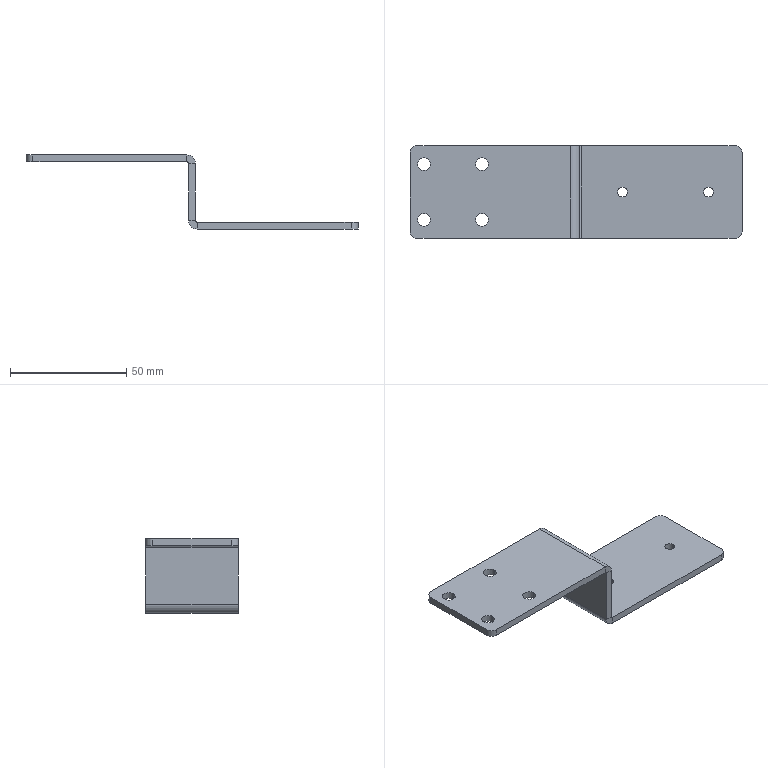Part | SolidWorks | features HoleWzd 2, Fillet 1, FlatPattern 1, SMBaseFlange 1, SheetMetal 1 | 1 solid | 38 faces | box 143 x 40 x 32 mm | volume 20017 mm3 | cylinder 20 | plane 18 | commonest cylinder face diameters 5.5 x8 4.2 x4 6 x4 1.5 x2 7.5 x2
STEP:
#1=CARTESIAN_POINT('',(8.75,8.,0.));
#2=VERTEX_POINT('',#1);
#3=CARTESIAN_POINT('',(3.25,8.,0.));
#4=VERTEX_POINT('',#3);
#5=CARTESIAN_POINT('',(6.,8.,0.));
#6=DIRECTION('',(0.,0.,-1.));
#7=DIRECTION('',(-1.,0.,0.));
#8=AXIS2_PLACEMENT_3D('',#5,#6,#7);
#9=CIRCLE('',#8,2.75);
#10=EDGE_CURVE('',#2,#4,#9,.T.);
#11=ORIENTED_EDGE('',*,*,#10,.T.);
#12=CARTESIAN_POINT('',(3.25,8.,3.));
#13=VERTEX_POINT('',#12);
#14=CARTESIAN_POINT('',(3.25,8.,3.));
#15=DIRECTION('',(0.,0.,1.));
#16=VECTOR('',#15,1000.);
#17=LINE('',#14,#16);
#18=EDGE_CURVE('',#4,#13,#17,.T.);
#19=ORIENTED_EDGE('',*,*,#18,.T.);
#20=CARTESIAN_POINT('',(8.75,8.,3.));
#21=VERTEX_POINT('',#20);
#22=CARTESIAN_POINT('',(6.,8.,3.));
#23=DIRECTION('',(0.,0.,1.));
#24=DIRECTION('',(1.,0.,0.));
#25=AXIS2_PLACEMENT_3D('',#22,#23,#24);
#26=CIRCLE('',#25,2.75);
#27=EDGE_CURVE('',#13,#21,#26,.T.);
#28=ORIENTED_EDGE('',*,*,#27,.T.);
#29=CARTESIAN_POINT('',(8.75,8.,3.));
#30=DIRECTION('',(0.,0.,1.));
#31=VECTOR('',#30,1000.);
#32=LINE('',#29,#31);
#33=EDGE_CURVE('',#2,#21,#32,.T.);
#34=ORIENTED_EDGE('',*,*,#33,.F.);
#35=EDGE_LOOP('',(#11,#19,#28,#34));
#36=FACE_OUTER_BOUND('',#35,.T.);
#37=CARTESIAN_POINT('',(6.,8.,3.));
#38=DIRECTION('',(0.,0.,1.));
#39=DIRECTION('',(1.,0.,0.));
#40=AXIS2_PLACEMENT_3D('',#37,#38,#39);
#41=CYLINDRICAL_SURFACE('',#40,2.75);
#42=ADVANCED_FACE('',(#36),#41,.F.);
#43=CARTESIAN_POINT('',(8.75,32.,0.));
#44=VERTEX_POINT('',#43);
#45=CARTESIAN_POINT('',(3.25,32.,0.));
#46=VERTEX_POINT('',#45);
#47=CARTESIAN_POINT('',(6.,32.,0.));
#48=DIRECTION('',(0.,0.,-1.));
#49=DIRECTION('',(-1.,0.,0.));
#50=AXIS2_PLACEMENT_3D('',#47,#48,#49);
#51=CIRCLE('',#50,2.75);
#52=EDGE_CURVE('',#44,#46,#51,.T.);
#53=ORIENTED_EDGE('',*,*,#52,.T.);
#54=CARTESIAN_POINT('',(3.25,32.,3.));
#55=VERTEX_POINT('',#54);
#56=CARTESIAN_POINT('',(3.25,32.,3.));
#57=DIRECTION('',(0.,0.,1.));
#58=VECTOR('',#57,1000.);
#59=LINE('',#56,#58);
#60=EDGE_CURVE('',#46,#55,#59,.T.);
#61=ORIENTED_EDGE('',*,*,#60,.T.);
#62=CARTESIAN_POINT('',(8.75,32.,3.));
#63=VERTEX_POINT('',#62);
#64=CARTESIAN_POINT('',(6.,32.,3.));
#65=DIRECTION('',(0.,0.,1.));
#66=DIRECTION('',(1.,0.,0.));
#67=AXIS2_PLACEMENT_3D('',#64,#65,#66);
#68=CIRCLE('',#67,2.75);
#69=EDGE_CURVE('',#55,#63,#68,.T.);
#70=ORIENTED_EDGE('',*,*,#69,.T.);
#71=CARTESIAN_POINT('',(8.75,32.,3.));
#72=DIRECTION('',(0.,0.,1.));
#73=VECTOR('',#72,1000.);
#74=LINE('',#71,#73);
#75=EDGE_CURVE('',#44,#63,#74,.T.);
#76=ORIENTED_EDGE('',*,*,#75,.F.);
#77=EDGE_LOOP('',(#53,#61,#70,#76));
#78=FACE_OUTER_BOUND('',#77,.T.);
#79=CARTESIAN_POINT('',(6.,32.,3.));
#80=DIRECTION('',(0.,0.,1.));
#81=DIRECTION('',(1.,0.,0.));
#82=AXIS2_PLACEMENT_3D('',#79,#80,#81);
#83=CYLINDRICAL_SURFACE('',#82,2.75);
#84=ADVANCED_FACE('',(#78),#83,.F.);
#85=CARTESIAN_POINT('',(33.75,8.,0.));
#86=VERTEX_POINT('',#85);
#87=CARTESIAN_POINT('',(28.25,8.,0.));
#88=VERTEX_POINT('',#87);
#89=CARTESIAN_POINT('',(31.,8.,0.));
#90=DIRECTION('',(0.,0.,-1.));
#91=DIRECTION('',(-1.,0.,0.));
#92=AXIS2_PLACEMENT_3D('',#89,#90,#91);
#93=CIRCLE('',#92,2.75);
#94=EDGE_CURVE('',#86,#88,#93,.T.);
#95=ORIENTED_EDGE('',*,*,#94,.T.);
#96=CARTESIAN_POINT('',(28.25,8.,3.));
#97=VERTEX_POINT('',#96);
#98=CARTESIAN_POINT('',(28.25,8.,3.));
#99=DIRECTION('',(0.,0.,1.));
#100=VECTOR('',#99,1000.);
#101=LINE('',#98,#100);
#102=EDGE_CURVE('',#88,#97,#101,.T.);
#103=ORIENTED_EDGE('',*,*,#102,.T.);
#104=CARTESIAN_POINT('',(33.75,8.,3.));
#105=VERTEX_POINT('',#104);
#106=CARTESIAN_POINT('',(31.,8.,3.));
#107=DIRECTION('',(0.,0.,1.));
#108=DIRECTION('',(1.,0.,0.));
#109=AXIS2_PLACEMENT_3D('',#106,#107,#108);
#110=CIRCLE('',#109,2.75);
#111=EDGE_CURVE('',#97,#105,#110,.T.);
#112=ORIENTED_EDGE('',*,*,#111,.T.);
#113=CARTESIAN_POINT('',(33.75,8.,3.));
#114=DIRECTION('',(0.,0.,1.));
#115=VECTOR('',#114,1000.);
#116=LINE('',#113,#115);
#117=EDGE_CURVE('',#86,#105,#116,.T.);
#118=ORIENTED_EDGE('',*,*,#117,.F.);
#119=EDGE_LOOP('',(#95,#103,#112,#118));
#120=FACE_OUTER_BOUND('',#119,.T.);
#121=CARTESIAN_POINT('',(31.,8.,3.));
#122=DIRECTION('',(0.,0.,1.));
#123=DIRECTION('',(1.,0.,0.));
#124=AXIS2_PLACEMENT_3D('',#121,#122,#123);
#125=CYLINDRICAL_SURFACE('',#124,2.75);
#126=ADVANCED_FACE('',(#120),#125,.F.);
#127=CARTESIAN_POINT('',(33.75,32.,0.));
#128=VERTEX_POINT('',#127);
#129=CARTESIAN_POINT('',(28.25,32.,0.));
#130=VERTEX_POINT('',#129);
#131=CARTESIAN_POINT('',(31.,32.,0.));
#132=DIRECTION('',(0.,0.,-1.));
#133=DIRECTION('',(-1.,0.,0.));
#134=AXIS2_PLACEMENT_3D('',#131,#132,#133);
#135=CIRCLE('',#134,2.75);
#136=EDGE_CURVE('',#128,#130,#135,.T.);
#137=ORIENTED_EDGE('',*,*,#136,.T.);
#138=CARTESIAN_POINT('',(28.25,32.,3.));
#139=VERTEX_POINT('',#138);
#140=CARTESIAN_POINT('',(28.25,32.,3.));
#141=DIRECTION('',(0.,0.,1.));
#142=VECTOR('',#141,1000.);
#143=LINE('',#140,#142);
#144=EDGE_CURVE('',#130,#139,#143,.T.);
#145=ORIENTED_EDGE('',*,*,#144,.T.);
#146=CARTESIAN_POINT('',(33.75,32.,3.));
#147=VERTEX_POINT('',#146);
#148=CARTESIAN_POINT('',(31.,32.,3.));
#149=DIRECTION('',(0.,0.,1.));
#150=DIRECTION('',(1.,0.,0.));
#151=AXIS2_PLACEMENT_3D('',#148,#149,#150);
#152=CIRCLE('',#151,2.75);
#153=EDGE_CURVE('',#139,#147,#152,.T.);
#154=ORIENTED_EDGE('',*,*,#153,.T.);
#155=CARTESIAN_POINT('',(33.75,32.,3.));
#156=DIRECTION('',(0.,0.,1.));
#157=VECTOR('',#156,1000.);
#158=LINE('',#155,#157);
#159=EDGE_CURVE('',#128,#147,#158,.T.);
#160=ORIENTED_EDGE('',*,*,#159,.F.);
#161=EDGE_LOOP('',(#137,#145,#154,#160));
#162=FACE_OUTER_BOUND('',#161,.T.);
#163=CARTESIAN_POINT('',(31.,32.,3.));
#164=DIRECTION('',(0.,0.,1.));
#165=DIRECTION('',(1.,0.,0.));
#166=AXIS2_PLACEMENT_3D('',#163,#164,#165);
#167=CYLINDRICAL_SURFACE('',#166,2.75);
#168=ADVANCED_FACE('',(#162),#167,.F.);
#169=CARTESIAN_POINT('',(130.65,20.,-29.));
#170=VERTEX_POINT('',#169);
#171=CARTESIAN_POINT('',(126.45,20.,-29.));
#172=VERTEX_POINT('',#171);
#173=CARTESIAN_POINT('',(128.55,20.,-29.));
#174=DIRECTION('',(0.,0.,-1.));
#175=DIRECTION('',(-1.,0.,0.));
#176=AXIS2_PLACEMENT_3D('',#173,#174,#175);
#177=CIRCLE('',#176,2.1);
#178=EDGE_CURVE('',#170,#172,#177,.T.);
#179=ORIENTED_EDGE('',*,*,#178,.T.);
#180=CARTESIAN_POINT('',(126.45,20.,-26.));
#181=VERTEX_POINT('',#180);
#182=CARTESIAN_POINT('',(126.45,20.,-26.));
#183=DIRECTION('',(0.,0.,1.));
#184=VECTOR('',#183,1000.);
#185=LINE('',#182,#184);
#186=EDGE_CURVE('',#172,#181,#185,.T.);
#187=ORIENTED_EDGE('',*,*,#186,.T.);
#188=CARTESIAN_POINT('',(130.65,20.,-26.));
#189=VERTEX_POINT('',#188);
#190=CARTESIAN_POINT('',(128.55,20.,-26.));
#191=DIRECTION('',(0.,0.,1.));
#192=DIRECTION('',(1.,0.,0.));
#193=AXIS2_PLACEMENT_3D('',#190,#191,#192);
#194=CIRCLE('',#193,2.1);
#195=EDGE_CURVE('',#181,#189,#194,.T.);
#196=ORIENTED_EDGE('',*,*,#195,.T.);
#197=CARTESIAN_POINT('',(130.65,20.,-26.));
#198=DIRECTION('',(0.,0.,1.));
#199=VECTOR('',#198,1000.);
#200=LINE('',#197,#199);
#201=EDGE_CURVE('',#170,#189,#200,.T.);
#202=ORIENTED_EDGE('',*,*,#201,.F.);
#203=EDGE_LOOP('',(#179,#187,#196,#202));
#204=FACE_OUTER_BOUND('',#203,.T.);
#205=CARTESIAN_POINT('',(128.55,20.,-26.));
#206=DIRECTION('',(0.,0.,1.));
#207=DIRECTION('',(1.,0.,0.));
#208=AXIS2_PLACEMENT_3D('',#205,#206,#207);
#209=CYLINDRICAL_SURFACE('',#208,2.1);
#210=ADVANCED_FACE('',(#204),#209,.F.);
#211=CARTESIAN_POINT('',(93.65,20.,-29.));
#212=VERTEX_POINT('',#211);
#213=CARTESIAN_POINT('',(89.45,20.,-29.));
#214=VERTEX_POINT('',#213);
#215=CARTESIAN_POINT('',(91.55,20.,-29.));
#216=DIRECTION('',(0.,0.,-1.));
#217=DIRECTION('',(-1.,0.,0.));
#218=AXIS2_PLACEMENT_3D('',#215,#216,#217);
#219=CIRCLE('',#218,2.1);
#220=EDGE_CURVE('',#212,#214,#219,.T.);
#221=ORIENTED_EDGE('',*,*,#220,.T.);
#222=CARTESIAN_POINT('',(89.45,20.,-26.));
#223=VERTEX_POINT('',#222);
#224=CARTESIAN_POINT('',(89.45,20.,-26.));
#225=DIRECTION('',(0.,0.,1.));
#226=VECTOR('',#225,1000.);
#227=LINE('',#224,#226);
#228=EDGE_CURVE('',#214,#223,#227,.T.);
#229=ORIENTED_EDGE('',*,*,#228,.T.);
#230=CARTESIAN_POINT('',(93.65,20.,-26.));
#231=VERTEX_POINT('',#230);
#232=CARTESIAN_POINT('',(91.55,20.,-26.));
#233=DIRECTION('',(0.,0.,1.));
#234=DIRECTION('',(1.,0.,0.));
#235=AXIS2_PLACEMENT_3D('',#232,#233,#234);
#236=CIRCLE('',#235,2.1);
#237=EDGE_CURVE('',#223,#231,#236,.T.);
#238=ORIENTED_EDGE('',*,*,#237,.T.);
#239=CARTESIAN_POINT('',(93.65,20.,-26.));
#240=DIRECTION('',(0.,0.,1.));
#241=VECTOR('',#240,1000.);
#242=LINE('',#239,#241);
#243=EDGE_CURVE('',#212,#231,#242,.T.);
#244=ORIENTED_EDGE('',*,*,#243,.F.);
#245=EDGE_LOOP('',(#221,#229,#238,#244));
#246=FACE_OUTER_BOUND('',#245,.T.);
#247=CARTESIAN_POINT('',(91.55,20.,-26.));
#248=DIRECTION('',(0.,0.,1.));
#249=DIRECTION('',(1.,0.,0.));
#250=AXIS2_PLACEMENT_3D('',#247,#248,#249);
#251=CYLINDRICAL_SURFACE('',#250,2.1);
#252=ADVANCED_FACE('',(#246),#251,.F.);
#253=CARTESIAN_POINT('',(70.,40.,-0.75));
#254=VERTEX_POINT('',#253);
#255=CARTESIAN_POINT('',(73.,40.,-0.75));
#256=VERTEX_POINT('',#255);
#257=CARTESIAN_POINT('',(70.,40.,-0.75));
#258=DIRECTION('',(1.,0.,0.));
#259=VECTOR('',#258,1000.);
#260=LINE('',#257,#259);
#261=EDGE_CURVE('',#254,#256,#260,.T.);
#262=ORIENTED_EDGE('',*,*,#261,.F.);
#263=CARTESIAN_POINT('',(69.25,40.,0.));
#264=VERTEX_POINT('',#263);
#265=CARTESIAN_POINT('',(69.25,40.,-0.75));
#266=DIRECTION('',(0.,1.,0.));
#267=DIRECTION('',(0.,0.,-1.));
#268=AXIS2_PLACEMENT_3D('',#265,#266,#267);
#269=CIRCLE('',#268,0.75);
#270=EDGE_CURVE('',#264,#254,#269,.T.);
#271=ORIENTED_EDGE('',*,*,#270,.F.);
#272=CARTESIAN_POINT('',(69.25,40.,3.));
#273=VERTEX_POINT('',#272);
#274=CARTESIAN_POINT('',(69.25,40.,3.));
#275=DIRECTION('',(0.,0.,-1.));
#276=VECTOR('',#275,1000.);
#277=LINE('',#274,#276);
#278=EDGE_CURVE('',#273,#264,#277,.T.);
#279=ORIENTED_EDGE('',*,*,#278,.F.);
#280=CARTESIAN_POINT('',(69.25,40.,-0.75));
#281=DIRECTION('',(0.,1.,0.));
#282=DIRECTION('',(1.,0.,0.));
#283=AXIS2_PLACEMENT_3D('',#280,#281,#282);
#284=CIRCLE('',#283,3.75);
#285=EDGE_CURVE('',#273,#256,#284,.T.);
#286=ORIENTED_EDGE('',*,*,#285,.T.);
#287=EDGE_LOOP('',(#262,#271,#279,#286));
#288=FACE_OUTER_BOUND('',#287,.T.);
#289=CARTESIAN_POINT('',(70.,40.,-0.75));
#290=DIRECTION('',(0.,1.,0.));
#291=DIRECTION('',(0.,0.,1.));
#292=AXIS2_PLACEMENT_3D('',#289,#290,#291);
#293=PLANE('',#292);
#294=ADVANCED_FACE('',(#288),#293,.T.);
#295=CARTESIAN_POINT('',(70.,40.,-25.25));
#296=VERTEX_POINT('',#295);
#297=CARTESIAN_POINT('',(70.,40.,0.));
#298=DIRECTION('',(0.,0.,-1.));
#299=VECTOR('',#298,1000.);
#300=LINE('',#297,#299);
#301=EDGE_CURVE('',#254,#296,#300,.T.);
#302=ORIENTED_EDGE('',*,*,#301,.F.);
#303=ORIENTED_EDGE('',*,*,#261,.T.);
#304=CARTESIAN_POINT('',(73.,40.,-25.25));
#305=VERTEX_POINT('',#304);
#306=CARTESIAN_POINT('',(73.,40.,0.));
#307=DIRECTION('',(0.,0.,-1.));
#308=VECTOR('',#307,1000.);
#309=LINE('',#306,#308);
#310=EDGE_CURVE('',#256,#305,#309,.T.);
#311=ORIENTED_EDGE('',*,*,#310,.T.);
#312=CARTESIAN_POINT('',(73.,40.,-25.25));
#313=DIRECTION('',(-1.,0.,0.));
#314=VECTOR('',#313,1000.);
#315=LINE('',#312,#314);
#316=EDGE_CURVE('',#305,#296,#315,.T.);
#317=ORIENTED_EDGE('',*,*,#316,.T.);
#318=EDGE_LOOP('',(#302,#303,#311,#317));
#319=FACE_OUTER_BOUND('',#318,.T.);
#320=CARTESIAN_POINT('',(69.25,40.,3.));
#321=DIRECTION('',(0.,1.,0.));
#322=DIRECTION('',(0.,0.,1.));
#323=AXIS2_PLACEMENT_3D('',#320,#321,#322);
#324=PLANE('',#323);
#325=ADVANCED_FACE('',(#319),#324,.T.);
#326=CARTESIAN_POINT('',(69.25,0.,0.));
#327=VERTEX_POINT('',#326);
#328=CARTESIAN_POINT('',(69.25,0.,3.));
#329=VERTEX_POINT('',#328);
#330=CARTESIAN_POINT('',(69.25,0.,0.));
#331=DIRECTION('',(0.,0.,1.));
#332=VECTOR('',#331,1000.);
#333=LINE('',#330,#332);
#334=EDGE_CURVE('',#327,#329,#333,.T.);
#335=ORIENTED_EDGE('',*,*,#334,.F.);
#336=CARTESIAN_POINT('',(70.,0.,-0.75));
#337=VERTEX_POINT('',#336);
#338=CARTESIAN_POINT('',(69.25,0.,-0.75));
#339=DIRECTION('',(0.,1.,0.));
#340=DIRECTION('',(0.,0.,-1.));
#341=AXIS2_PLACEMENT_3D('',#338,#339,#340);
#342=CIRCLE('',#341,0.75);
#343=EDGE_CURVE('',#327,#337,#342,.T.);
#344=ORIENTED_EDGE('',*,*,#343,.T.);
#345=CARTESIAN_POINT('',(73.,0.,-0.75));
#346=VERTEX_POINT('',#345);
#347=CARTESIAN_POINT('',(73.,0.,-0.75));
#348=DIRECTION('',(-1.,0.,0.));
#349=VECTOR('',#348,1000.);
#350=LINE('',#347,#349);
#351=EDGE_CURVE('',#346,#337,#350,.T.);
#352=ORIENTED_EDGE('',*,*,#351,.F.);
#353=CARTESIAN_POINT('',(69.25,0.,-0.75));
#354=DIRECTION('',(0.,1.,0.));
#355=DIRECTION('',(1.,0.,0.));
#356=AXIS2_PLACEMENT_3D('',#353,#354,#355);
#357=CIRCLE('',#356,3.75);
#358=EDGE_CURVE('',#329,#346,#357,.T.);
#359=ORIENTED_EDGE('',*,*,#358,.F.);
#360=EDGE_LOOP('',(#335,#344,#352,#359));
#361=FACE_OUTER_BOUND('',#360,.T.);
#362=CARTESIAN_POINT('',(69.25,0.,0.));
#363=DIRECTION('',(0.,-1.,0.));
#364=DIRECTION('',(0.,0.,-1.));
#365=AXIS2_PLACEMENT_3D('',#362,#363,#364);
#366=PLANE('',#365);
#367=ADVANCED_FACE('',(#361),#366,.T.);
#368=CARTESIAN_POINT('',(3.,0.,3.));
#369=VERTEX_POINT('',#368);
#370=CARTESIAN_POINT('',(0.,0.,3.));
#371=DIRECTION('',(1.,0.,0.));
#372=VECTOR('',#371,1000.);
#373=LINE('',#370,#372);
#374=EDGE_CURVE('',#369,#329,#373,.T.);
#375=ORIENTED_EDGE('',*,*,#374,.F.);
#376=CARTESIAN_POINT('',(3.,0.,0.));
#377=VERTEX_POINT('',#376);
#378=CARTESIAN_POINT('',(3.,0.,-0.75));
#379=DIRECTION('',(0.,0.,-1.));
#380=VECTOR('',#379,1000.);
#381=LINE('',#378,#380);
#382=EDGE_CURVE('',#369,#377,#381,.T.);
#383=ORIENTED_EDGE('',*,*,#382,.T.);
#384=CARTESIAN_POINT('',(0.,0.,0.));
#385=DIRECTION('',(1.,0.,0.));
#386=VECTOR('',#385,1000.);
#387=LINE('',#384,#386);
#388=EDGE_CURVE('',#377,#327,#387,.T.);
#389=ORIENTED_EDGE('',*,*,#388,.T.);
#390=ORIENTED_EDGE('',*,*,#334,.T.);
#391=EDGE_LOOP('',(#375,#383,#389,#390));
#392=FACE_OUTER_BOUND('',#391,.T.);
#393=CARTESIAN_POINT('',(73.,0.,-0.75));
#394=DIRECTION('',(0.,-1.,0.));
#395=DIRECTION('',(0.,0.,-1.));
#396=AXIS2_PLACEMENT_3D('',#393,#394,#395);
#397=PLANE('',#396);
#398=ADVANCED_FACE('',(#392),#397,.T.);
#399=CARTESIAN_POINT('',(73.75,40.,-29.));
#400=VERTEX_POINT('',#399);
#401=CARTESIAN_POINT('',(73.75,40.,-26.));
#402=VERTEX_POINT('',#401);
#403=CARTESIAN_POINT('',(73.75,40.,-29.));
#404=DIRECTION('',(0.,0.,1.));
#405=VECTOR('',#404,1000.);
#406=LINE('',#403,#405);
#407=EDGE_CURVE('',#400,#402,#406,.T.);
#408=ORIENTED_EDGE('',*,*,#407,.F.);
#409=CARTESIAN_POINT('',(73.75,40.,-25.25));
#410=DIRECTION('',(0.,-1.,0.));
#411=DIRECTION('',(0.,0.,1.));
#412=AXIS2_PLACEMENT_3D('',#409,#410,#411);
#413=CIRCLE('',#412,3.75);
#414=EDGE_CURVE('',#296,#400,#413,.T.);
#415=ORIENTED_EDGE('',*,*,#414,.F.);
#416=ORIENTED_EDGE('',*,*,#316,.F.);
#417=CARTESIAN_POINT('',(73.75,40.,-25.25));
#418=DIRECTION('',(0.,-1.,0.));
#419=DIRECTION('',(1.,0.,0.));
#420=AXIS2_PLACEMENT_3D('',#417,#418,#419);
#421=CIRCLE('',#420,0.75);
#422=EDGE_CURVE('',#305,#402,#421,.T.);
#423=ORIENTED_EDGE('',*,*,#422,.T.);
#424=EDGE_LOOP('',(#408,#415,#416,#423));
#425=FACE_OUTER_BOUND('',#424,.T.);
#426=CARTESIAN_POINT('',(73.75,40.,-29.));
#427=DIRECTION('',(0.,1.,0.));
#428=DIRECTION('',(0.,0.,1.));
#429=AXIS2_PLACEMENT_3D('',#426,#427,#428);
#430=PLANE('',#429);
#431=ADVANCED_FACE('',(#425),#430,.T.);
#432=CARTESIAN_POINT('',(140.,40.,-26.));
#433=VERTEX_POINT('',#432);
#434=CARTESIAN_POINT('',(70.,40.,-26.));
#435=DIRECTION('',(1.,0.,0.));
#436=VECTOR('',#435,1000.);
#437=LINE('',#434,#436);
#438=EDGE_CURVE('',#402,#433,#437,.T.);
#439=ORIENTED_EDGE('',*,*,#438,.T.);
#440=CARTESIAN_POINT('',(140.,40.,-29.));
#441=VERTEX_POINT('',#440);
#442=CARTESIAN_POINT('',(140.,40.,-25.25));
#443=DIRECTION('',(0.,0.,-1.));
#444=VECTOR('',#443,1000.);
#445=LINE('',#442,#444);
#446=EDGE_CURVE('',#433,#441,#445,.T.);
#447=ORIENTED_EDGE('',*,*,#446,.T.);
#448=CARTESIAN_POINT('',(70.,40.,-29.));
#449=DIRECTION('',(1.,0.,0.));
#450=VECTOR('',#449,1000.);
#451=LINE('',#448,#450);
#452=EDGE_CURVE('',#400,#441,#451,.T.);
#453=ORIENTED_EDGE('',*,*,#452,.F.);
#454=ORIENTED_EDGE('',*,*,#407,.T.);
#455=EDGE_LOOP('',(#439,#447,#453,#454));
#456=FACE_OUTER_BOUND('',#455,.T.);
#457=CARTESIAN_POINT('',(73.,40.,-25.25));
#458=DIRECTION('',(0.,1.,0.));
#459=DIRECTION('',(0.,0.,1.));
#460=AXIS2_PLACEMENT_3D('',#457,#458,#459);
#461=PLANE('',#460);
#462=ADVANCED_FACE('',(#456),#461,.T.);
#463=CARTESIAN_POINT('',(70.,0.,-25.25));
#464=VERTEX_POINT('',#463);
#465=CARTESIAN_POINT('',(73.,0.,-25.25));
#466=VERTEX_POINT('',#465);
#467=CARTESIAN_POINT('',(70.,0.,-25.25));
#468=DIRECTION('',(1.,0.,0.));
#469=VECTOR('',#468,1000.);
#470=LINE('',#467,#469);
#471=EDGE_CURVE('',#464,#466,#470,.T.);
#472=ORIENTED_EDGE('',*,*,#471,.F.);
#473=CARTESIAN_POINT('',(73.75,0.,-29.));
#474=VERTEX_POINT('',#473);
#475=CARTESIAN_POINT('',(73.75,0.,-25.25));
#476=DIRECTION('',(0.,-1.,0.));
#477=DIRECTION('',(0.,0.,1.));
#478=AXIS2_PLACEMENT_3D('',#475,#476,#477);
#479=CIRCLE('',#478,3.75);
#480=EDGE_CURVE('',#464,#474,#479,.T.);
#481=ORIENTED_EDGE('',*,*,#480,.T.);
#482=CARTESIAN_POINT('',(73.75,0.,-26.));
#483=VERTEX_POINT('',#482);
#484=CARTESIAN_POINT('',(73.75,0.,-26.));
#485=DIRECTION('',(0.,0.,-1.));
#486=VECTOR('',#485,1000.);
#487=LINE('',#484,#486);
#488=EDGE_CURVE('',#483,#474,#487,.T.);
#489=ORIENTED_EDGE('',*,*,#488,.F.);
#490=CARTESIAN_POINT('',(73.75,0.,-25.25));
#491=DIRECTION('',(0.,-1.,0.));
#492=DIRECTION('',(1.,0.,0.));
#493=AXIS2_PLACEMENT_3D('',#490,#491,#492);
#494=CIRCLE('',#493,0.75);
#495=EDGE_CURVE('',#466,#483,#494,.T.);
#496=ORIENTED_EDGE('',*,*,#495,.F.);
#497=EDGE_LOOP('',(#472,#481,#489,#496));
#498=FACE_OUTER_BOUND('',#497,.T.);
#499=CARTESIAN_POINT('',(70.,0.,-25.25));
#500=DIRECTION('',(0.,-1.,0.));
#501=DIRECTION('',(0.,0.,-1.));
#502=AXIS2_PLACEMENT_3D('',#499,#500,#501);
#503=PLANE('',#502);
#504=ADVANCED_FACE('',(#498),#503,.T.);
#505=CARTESIAN_POINT('',(70.,0.,0.));
#506=DIRECTION('',(0.,0.,-1.));
#507=VECTOR('',#506,1000.);
#508=LINE('',#505,#507);
#509=EDGE_CURVE('',#337,#464,#508,.T.);
#510=ORIENTED_EDGE('',*,*,#509,.T.);
#511=ORIENTED_EDGE('',*,*,#471,.T.);
#512=CARTESIAN_POINT('',(73.,0.,0.));
#513=DIRECTION('',(0.,0.,-1.));
#514=VECTOR('',#513,1000.);
#515=LINE('',#512,#514);
#516=EDGE_CURVE('',#346,#466,#515,.T.);
#517=ORIENTED_EDGE('',*,*,#516,.F.);
#518=ORIENTED_EDGE('',*,*,#351,.T.);
#519=EDGE_LOOP('',(#510,#511,#517,#518));
#520=FACE_OUTER_BOUND('',#519,.T.);
#521=CARTESIAN_POINT('',(73.75,0.,-26.));
#522=DIRECTION('',(0.,-1.,0.));
#523=DIRECTION('',(0.,0.,-1.));
#524=AXIS2_PLACEMENT_3D('',#521,#522,#523);
#525=PLANE('',#524);
#526=ADVANCED_FACE('',(#520),#525,.T.);
#527=CARTESIAN_POINT('',(128.55,20.,-26.));
#528=DIRECTION('',(0.,0.,1.));
#529=DIRECTION('',(1.,0.,0.));
#530=AXIS2_PLACEMENT_3D('',#527,#528,#529);
#531=CIRCLE('',#530,2.1);
#532=EDGE_CURVE('',#189,#181,#531,.T.);
#533=ORIENTED_EDGE('',*,*,#532,.F.);
#534=ORIENTED_EDGE('',*,*,#195,.F.);
#535=EDGE_LOOP('',(#533,#534));
#536=FACE_BOUND('',#535,.T.);
#537=CARTESIAN_POINT('',(91.55,20.,-26.));
#538=DIRECTION('',(0.,0.,1.));
#539=DIRECTION('',(1.,0.,0.));
#540=AXIS2_PLACEMENT_3D('',#537,#538,#539);
#541=CIRCLE('',#540,2.1);
#542=EDGE_CURVE('',#231,#223,#541,.T.);
#543=ORIENTED_EDGE('',*,*,#542,.F.);
#544=ORIENTED_EDGE('',*,*,#237,.F.);
#545=EDGE_LOOP('',(#543,#544));
#546=FACE_BOUND('',#545,.T.);
#547=CARTESIAN_POINT('',(140.,0.,-26.));
#548=VERTEX_POINT('',#547);
#549=CARTESIAN_POINT('',(70.,0.,-26.));
#550=DIRECTION('',(1.,0.,0.));
#551=VECTOR('',#550,1000.);
#552=LINE('',#549,#551);
#553=EDGE_CURVE('',#483,#548,#552,.T.);
#554=ORIENTED_EDGE('',*,*,#553,.T.);
#555=CARTESIAN_POINT('',(143.,3.,-26.));
#556=VERTEX_POINT('',#555);
#557=CARTESIAN_POINT('',(140.,3.,-26.));
#558=DIRECTION('',(0.,0.,1.));
#559=DIRECTION('',(-1.,0.,0.));
#560=AXIS2_PLACEMENT_3D('',#557,#558,#559);
#561=CIRCLE('',#560,3.);
#562=EDGE_CURVE('',#548,#556,#561,.T.);
#563=ORIENTED_EDGE('',*,*,#562,.T.);
#564=CARTESIAN_POINT('',(143.,37.,-26.));
#565=VERTEX_POINT('',#564);
#566=CARTESIAN_POINT('',(143.,40.,-26.));
#567=DIRECTION('',(0.,-1.,0.));
#568=VECTOR('',#567,1000.);
#569=LINE('',#566,#568);
#570=EDGE_CURVE('',#565,#556,#569,.T.);
#571=ORIENTED_EDGE('',*,*,#570,.F.);
#572=CARTESIAN_POINT('',(140.,37.,-26.));
#573=DIRECTION('',(0.,0.,1.));
#574=DIRECTION('',(-1.,0.,0.));
#575=AXIS2_PLACEMENT_3D('',#572,#573,#574);
#576=CIRCLE('',#575,3.);
#577=EDGE_CURVE('',#565,#433,#576,.T.);
#578=ORIENTED_EDGE('',*,*,#577,.T.);
#579=ORIENTED_EDGE('',*,*,#438,.F.);
#580=CARTESIAN_POINT('',(73.75,40.,-26.));
#581=DIRECTION('',(0.,-1.,0.));
#582=VECTOR('',#581,1000.);
#583=LINE('',#580,#582);
#584=EDGE_CURVE('',#402,#483,#583,.T.);
#585=ORIENTED_EDGE('',*,*,#584,.T.);
#586=EDGE_LOOP('',(#554,#563,#571,#578,#579,#585));
#587=FACE_OUTER_BOUND('',#586,.T.);
#588=CARTESIAN_POINT('',(70.,40.,-26.));
#589=DIRECTION('',(0.,0.,-1.));
#590=DIRECTION('',(-1.,0.,0.));
#591=AXIS2_PLACEMENT_3D('',#588,#589,#590);
#592=PLANE('',#591);
#593=ADVANCED_FACE('',(#536,#546,#587),#592,.F.);
#594=ORIENTED_EDGE('',*,*,#570,.T.);
#595=CARTESIAN_POINT('',(143.,3.,-29.));
#596=VERTEX_POINT('',#595);
#597=CARTESIAN_POINT('',(143.,3.,-29.));
#598=DIRECTION('',(0.,0.,-1.));
#599=VECTOR('',#598,1000.);
#600=LINE('',#597,#599);
#601=EDGE_CURVE('',#556,#596,#600,.T.);
#602=ORIENTED_EDGE('',*,*,#601,.T.);
#603=CARTESIAN_POINT('',(143.,37.,-29.));
#604=VERTEX_POINT('',#603);
#605=CARTESIAN_POINT('',(143.,40.,-29.));
#606=DIRECTION('',(0.,-1.,0.));
#607=VECTOR('',#606,1000.);
#608=LINE('',#605,#607);
#609=EDGE_CURVE('',#604,#596,#608,.T.);
#610=ORIENTED_EDGE('',*,*,#609,.F.);
#611=CARTESIAN_POINT('',(143.,37.,-29.));
#612=DIRECTION('',(0.,0.,1.));
#613=VECTOR('',#612,1000.);
#614=LINE('',#611,#613);
#615=EDGE_CURVE('',#604,#565,#614,.T.);
#616=ORIENTED_EDGE('',*,*,#615,.T.);
#617=EDGE_LOOP('',(#594,#602,#610,#616));
#618=FACE_OUTER_BOUND('',#617,.T.);
#619=CARTESIAN_POINT('',(143.,40.,-29.));
#620=DIRECTION('',(1.,0.,0.));
#621=DIRECTION('',(0.,0.,-1.));
#622=AXIS2_PLACEMENT_3D('',#619,#620,#621);
#623=PLANE('',#622);
#624=ADVANCED_FACE('',(#618),#623,.T.);
#625=ORIENTED_EDGE('',*,*,#178,.F.);
#626=CARTESIAN_POINT('',(128.55,20.,-29.));
#627=DIRECTION('',(0.,0.,-1.));
#628=DIRECTION('',(-1.,0.,0.));
#629=AXIS2_PLACEMENT_3D('',#626,#627,#628);
#630=CIRCLE('',#629,2.1);
#631=EDGE_CURVE('',#172,#170,#630,.T.);
#632=ORIENTED_EDGE('',*,*,#631,.F.);
#633=EDGE_LOOP('',(#625,#632));
#634=FACE_BOUND('',#633,.T.);
#635=ORIENTED_EDGE('',*,*,#220,.F.);
#636=CARTESIAN_POINT('',(91.55,20.,-29.));
#637=DIRECTION('',(0.,0.,-1.));
#638=DIRECTION('',(-1.,0.,0.));
#639=AXIS2_PLACEMENT_3D('',#636,#637,#638);
#640=CIRCLE('',#639,2.1);
#641=EDGE_CURVE('',#214,#212,#640,.T.);
#642=ORIENTED_EDGE('',*,*,#641,.F.);
#643=EDGE_LOOP('',(#635,#642));
#644=FACE_BOUND('',#643,.T.);
#645=ORIENTED_EDGE('',*,*,#609,.T.);
#646=CARTESIAN_POINT('',(140.,0.,-29.));
#647=VERTEX_POINT('',#646);
#648=CARTESIAN_POINT('',(140.,3.,-29.));
#649=DIRECTION('',(0.,0.,-1.));
#650=DIRECTION('',(-1.,0.,0.));
#651=AXIS2_PLACEMENT_3D('',#648,#649,#650);
#652=CIRCLE('',#651,3.);
#653=EDGE_CURVE('',#596,#647,#652,.T.);
#654=ORIENTED_EDGE('',*,*,#653,.T.);
#655=CARTESIAN_POINT('',(70.,0.,-29.));
#656=DIRECTION('',(1.,0.,0.));
#657=VECTOR('',#656,1000.);
#658=LINE('',#655,#657);
#659=EDGE_CURVE('',#474,#647,#658,.T.);
#660=ORIENTED_EDGE('',*,*,#659,.F.);
#661=CARTESIAN_POINT('',(73.75,40.,-29.));
#662=DIRECTION('',(0.,-1.,0.));
#663=VECTOR('',#662,1000.);
#664=LINE('',#661,#663);
#665=EDGE_CURVE('',#400,#474,#664,.T.);
#666=ORIENTED_EDGE('',*,*,#665,.F.);
#667=ORIENTED_EDGE('',*,*,#452,.T.);
#668=CARTESIAN_POINT('',(140.,37.,-29.));
#669=DIRECTION('',(0.,0.,-1.));
#670=DIRECTION('',(-1.,0.,0.));
#671=AXIS2_PLACEMENT_3D('',#668,#669,#670);
#672=CIRCLE('',#671,3.);
#673=EDGE_CURVE('',#441,#604,#672,.T.);
#674=ORIENTED_EDGE('',*,*,#673,.T.);
#675=EDGE_LOOP('',(#645,#654,#660,#666,#667,#674));
#676=FACE_OUTER_BOUND('',#675,.T.);
#677=CARTESIAN_POINT('',(70.,40.,-29.));
#678=DIRECTION('',(0.,0.,-1.));
#679=DIRECTION('',(-1.,0.,0.));
#680=AXIS2_PLACEMENT_3D('',#677,#678,#679);
#681=PLANE('',#680);
#682=ADVANCED_FACE('',(#634,#644,#676),#681,.T.);
#683=ORIENTED_EDGE('',*,*,#480,.F.);
#684=CARTESIAN_POINT('',(70.,40.,-25.25));
#685=DIRECTION('',(0.,-1.,0.));
#686=VECTOR('',#685,1000.);
#687=LINE('',#684,#686);
#688=EDGE_CURVE('',#296,#464,#687,.T.);
#689=ORIENTED_EDGE('',*,*,#688,.F.);
#690=ORIENTED_EDGE('',*,*,#414,.T.);
#691=ORIENTED_EDGE('',*,*,#665,.T.);
#692=EDGE_LOOP('',(#683,#689,#690,#691));
#693=FACE_OUTER_BOUND('',#692,.T.);
#694=CARTESIAN_POINT('',(73.75,40.,-25.25));
#695=DIRECTION('',(0.,-1.,0.));
#696=DIRECTION('',(0.,0.,-1.));
#697=AXIS2_PLACEMENT_3D('',#694,#695,#696);
#698=CYLINDRICAL_SURFACE('',#697,3.75);
#699=ADVANCED_FACE('',(#693),#698,.T.);
#700=ORIENTED_EDGE('',*,*,#509,.F.);
#701=CARTESIAN_POINT('',(70.,40.,-0.75));
#702=DIRECTION('',(0.,-1.,0.));
#703=VECTOR('',#702,1000.);
#704=LINE('',#701,#703);
#705=EDGE_CURVE('',#254,#337,#704,.T.);
#706=ORIENTED_EDGE('',*,*,#705,.F.);
#707=ORIENTED_EDGE('',*,*,#301,.T.);
#708=ORIENTED_EDGE('',*,*,#688,.T.);
#709=EDGE_LOOP('',(#700,#706,#707,#708));
#710=FACE_OUTER_BOUND('',#709,.T.);
#711=CARTESIAN_POINT('',(70.,40.,0.));
#712=DIRECTION('',(-1.,0.,0.));
#713=DIRECTION('',(0.,0.,1.));
#714=AXIS2_PLACEMENT_3D('',#711,#712,#713);
#715=PLANE('',#714);
#716=ADVANCED_FACE('',(#710),#715,.T.);
#717=ORIENTED_EDGE('',*,*,#343,.F.);
#718=CARTESIAN_POINT('',(69.25,40.,0.));
#719=DIRECTION('',(0.,-1.,0.));
#720=VECTOR('',#719,1000.);
#721=LINE('',#718,#720);
#722=EDGE_CURVE('',#264,#327,#721,.T.);
#723=ORIENTED_EDGE('',*,*,#722,.F.);
#724=ORIENTED_EDGE('',*,*,#270,.T.);
#725=ORIENTED_EDGE('',*,*,#705,.T.);
#726=EDGE_LOOP('',(#717,#723,#724,#725));
#727=FACE_OUTER_BOUND('',#726,.T.);
#728=CARTESIAN_POINT('',(69.25,40.,-0.75));
#729=DIRECTION('',(0.,-1.,0.));
#730=DIRECTION('',(0.,0.,-1.));
#731=AXIS2_PLACEMENT_3D('',#728,#729,#730);
#732=CYLINDRICAL_SURFACE('',#731,0.75);
#733=ADVANCED_FACE('',(#727),#732,.F.);
#734=ORIENTED_EDGE('',*,*,#10,.F.);
#735=CARTESIAN_POINT('',(6.,8.,0.));
#736=DIRECTION('',(0.,0.,-1.));
#737=DIRECTION('',(-1.,0.,0.));
#738=AXIS2_PLACEMENT_3D('',#735,#736,#737);
#739=CIRCLE('',#738,2.75);
#740=EDGE_CURVE('',#4,#2,#739,.T.);
#741=ORIENTED_EDGE('',*,*,#740,.F.);
#742=EDGE_LOOP('',(#734,#741));
#743=FACE_BOUND('',#742,.T.);
#744=ORIENTED_EDGE('',*,*,#52,.F.);
#745=CARTESIAN_POINT('',(6.,32.,0.));
#746=DIRECTION('',(0.,0.,-1.));
#747=DIRECTION('',(-1.,0.,0.));
#748=AXIS2_PLACEMENT_3D('',#745,#746,#747);
#749=CIRCLE('',#748,2.75);
#750=EDGE_CURVE('',#46,#44,#749,.T.);
#751=ORIENTED_EDGE('',*,*,#750,.F.);
#752=EDGE_LOOP('',(#744,#751));
#753=FACE_BOUND('',#752,.T.);
#754=ORIENTED_EDGE('',*,*,#94,.F.);
#755=CARTESIAN_POINT('',(31.,8.,0.));
#756=DIRECTION('',(0.,0.,-1.));
#757=DIRECTION('',(-1.,0.,0.));
#758=AXIS2_PLACEMENT_3D('',#755,#756,#757);
#759=CIRCLE('',#758,2.75);
#760=EDGE_CURVE('',#88,#86,#759,.T.);
#761=ORIENTED_EDGE('',*,*,#760,.F.);
#762=EDGE_LOOP('',(#754,#761));
#763=FACE_BOUND('',#762,.T.);
#764=ORIENTED_EDGE('',*,*,#136,.F.);
#765=CARTESIAN_POINT('',(31.,32.,0.));
#766=DIRECTION('',(0.,0.,-1.));
#767=DIRECTION('',(-1.,0.,0.));
#768=AXIS2_PLACEMENT_3D('',#765,#766,#767);
#769=CIRCLE('',#768,2.75);
#770=EDGE_CURVE('',#130,#128,#769,.T.);
#771=ORIENTED_EDGE('',*,*,#770,.F.);
#772=EDGE_LOOP('',(#764,#771));
#773=FACE_BOUND('',#772,.T.);
#774=ORIENTED_EDGE('',*,*,#388,.F.);
#775=CARTESIAN_POINT('',(0.,3.,0.));
#776=VERTEX_POINT('',#775);
#777=CARTESIAN_POINT('',(3.,3.,0.));
#778=DIRECTION('',(0.,0.,-1.));
#779=DIRECTION('',(-1.,0.,0.));
#780=AXIS2_PLACEMENT_3D('',#777,#778,#779);
#781=CIRCLE('',#780,3.);
#782=EDGE_CURVE('',#377,#776,#781,.T.);
#783=ORIENTED_EDGE('',*,*,#782,.T.);
#784=CARTESIAN_POINT('',(0.,37.,0.));
#785=VERTEX_POINT('',#784);
#786=CARTESIAN_POINT('',(0.,40.,0.));
#787=DIRECTION('',(0.,-1.,0.));
#788=VECTOR('',#787,1000.);
#789=LINE('',#786,#788);
#790=EDGE_CURVE('',#785,#776,#789,.T.);
#791=ORIENTED_EDGE('',*,*,#790,.F.);
#792=CARTESIAN_POINT('',(3.,40.,0.));
#793=VERTEX_POINT('',#792);
#794=CARTESIAN_POINT('',(3.,37.,0.));
#795=DIRECTION('',(0.,0.,-1.));
#796=DIRECTION('',(-1.,0.,0.));
#797=AXIS2_PLACEMENT_3D('',#794,#795,#796);
#798=CIRCLE('',#797,3.);
#799=EDGE_CURVE('',#785,#793,#798,.T.);
#800=ORIENTED_EDGE('',*,*,#799,.T.);
#801=CARTESIAN_POINT('',(0.,40.,0.));
#802=DIRECTION('',(1.,0.,0.));
#803=VECTOR('',#802,1000.);
#804=LINE('',#801,#803);
#805=EDGE_CURVE('',#793,#264,#804,.T.);
#806=ORIENTED_EDGE('',*,*,#805,.T.);
#807=ORIENTED_EDGE('',*,*,#722,.T.);
#808=EDGE_LOOP('',(#774,#783,#791,#800,#806,#807));
#809=FACE_OUTER_BOUND('',#808,.T.);
#810=CARTESIAN_POINT('',(0.,40.,0.));
#811=DIRECTION('',(0.,0.,-1.));
#812=DIRECTION('',(-1.,0.,0.));
#813=AXIS2_PLACEMENT_3D('',#810,#811,#812);
#814=PLANE('',#813);
#815=ADVANCED_FACE('',(#743,#753,#763,#773,#809),#814,.T.);
#816=ORIENTED_EDGE('',*,*,#790,.T.);
#817=CARTESIAN_POINT('',(0.,3.,3.));
#818=VERTEX_POINT('',#817);
#819=CARTESIAN_POINT('',(0.,3.,3.));
#820=DIRECTION('',(0.,0.,1.));
#821=VECTOR('',#820,1000.);
#822=LINE('',#819,#821);
#823=EDGE_CURVE('',#776,#818,#822,.T.);
#824=ORIENTED_EDGE('',*,*,#823,.T.);
#825=CARTESIAN_POINT('',(0.,37.,3.));
#826=VERTEX_POINT('',#825);
#827=CARTESIAN_POINT('',(0.,40.,3.));
#828=DIRECTION('',(0.,-1.,0.));
#829=VECTOR('',#828,1000.);
#830=LINE('',#827,#829);
#831=EDGE_CURVE('',#826,#818,#830,.T.);
#832=ORIENTED_EDGE('',*,*,#831,.F.);
#833=CARTESIAN_POINT('',(0.,37.,3.));
#834=DIRECTION('',(0.,0.,-1.));
#835=VECTOR('',#834,1000.);
#836=LINE('',#833,#835);
#837=EDGE_CURVE('',#826,#785,#836,.T.);
#838=ORIENTED_EDGE('',*,*,#837,.T.);
#839=EDGE_LOOP('',(#816,#824,#832,#838));
#840=FACE_OUTER_BOUND('',#839,.T.);
#841=CARTESIAN_POINT('',(0.,40.,3.));
#842=DIRECTION('',(-1.,0.,0.));
#843=DIRECTION('',(0.,0.,1.));
#844=AXIS2_PLACEMENT_3D('',#841,#842,#843);
#845=PLANE('',#844);
#846=ADVANCED_FACE('',(#840),#845,.T.);
#847=CARTESIAN_POINT('',(6.,8.,3.));
#848=DIRECTION('',(0.,0.,1.));
#849=DIRECTION('',(1.,0.,0.));
#850=AXIS2_PLACEMENT_3D('',#847,#848,#849);
#851=CIRCLE('',#850,2.75);
#852=EDGE_CURVE('',#21,#13,#851,.T.);
#853=ORIENTED_EDGE('',*,*,#852,.F.);
#854=ORIENTED_EDGE('',*,*,#27,.F.);
#855=EDGE_LOOP('',(#853,#854));
#856=FACE_BOUND('',#855,.T.);
#857=CARTESIAN_POINT('',(6.,32.,3.));
#858=DIRECTION('',(0.,0.,1.));
#859=DIRECTION('',(1.,0.,0.));
#860=AXIS2_PLACEMENT_3D('',#857,#858,#859);
#861=CIRCLE('',#860,2.75);
#862=EDGE_CURVE('',#63,#55,#861,.T.);
#863=ORIENTED_EDGE('',*,*,#862,.F.);
#864=ORIENTED_EDGE('',*,*,#69,.F.);
#865=EDGE_LOOP('',(#863,#864));
#866=FACE_BOUND('',#865,.T.);
#867=CARTESIAN_POINT('',(31.,8.,3.));
#868=DIRECTION('',(0.,0.,1.));
#869=DIRECTION('',(1.,0.,0.));
#870=AXIS2_PLACEMENT_3D('',#867,#868,#869);
#871=CIRCLE('',#870,2.75);
#872=EDGE_CURVE('',#105,#97,#871,.T.);
#873=ORIENTED_EDGE('',*,*,#872,.F.);
#874=ORIENTED_EDGE('',*,*,#111,.F.);
#875=EDGE_LOOP('',(#873,#874));
#876=FACE_BOUND('',#875,.T.);
#877=CARTESIAN_POINT('',(31.,32.,3.));
#878=DIRECTION('',(0.,0.,1.));
#879=DIRECTION('',(1.,0.,0.));
#880=AXIS2_PLACEMENT_3D('',#877,#878,#879);
#881=CIRCLE('',#880,2.75);
#882=EDGE_CURVE('',#147,#139,#881,.T.);
#883=ORIENTED_EDGE('',*,*,#882,.F.);
#884=ORIENTED_EDGE('',*,*,#153,.F.);
#885=EDGE_LOOP('',(#883,#884));
#886=FACE_BOUND('',#885,.T.);
#887=ORIENTED_EDGE('',*,*,#831,.T.);
#888=CARTESIAN_POINT('',(3.,3.,3.));
#889=DIRECTION('',(0.,0.,1.));
#890=DIRECTION('',(-1.,0.,0.));
#891=AXIS2_PLACEMENT_3D('',#888,#889,#890);
#892=CIRCLE('',#891,3.);
#893=EDGE_CURVE('',#818,#369,#892,.T.);
#894=ORIENTED_EDGE('',*,*,#893,.T.);
#895=ORIENTED_EDGE('',*,*,#374,.T.);
#896=CARTESIAN_POINT('',(69.25,40.,3.));
#897=DIRECTION('',(0.,-1.,0.));
#898=VECTOR('',#897,1000.);
#899=LINE('',#896,#898);
#900=EDGE_CURVE('',#273,#329,#899,.T.);
#901=ORIENTED_EDGE('',*,*,#900,.F.);
#902=CARTESIAN_POINT('',(3.,40.,3.));
#903=VERTEX_POINT('',#902);
#904=CARTESIAN_POINT('',(0.,40.,3.));
#905=DIRECTION('',(1.,0.,0.));
#906=VECTOR('',#905,1000.);
#907=LINE('',#904,#906);
#908=EDGE_CURVE('',#903,#273,#907,.T.);
#909=ORIENTED_EDGE('',*,*,#908,.F.);
#910=CARTESIAN_POINT('',(3.,37.,3.));
#911=DIRECTION('',(0.,0.,1.));
#912=DIRECTION('',(-1.,0.,0.));
#913=AXIS2_PLACEMENT_3D('',#910,#911,#912);
#914=CIRCLE('',#913,3.);
#915=EDGE_CURVE('',#903,#826,#914,.T.);
#916=ORIENTED_EDGE('',*,*,#915,.T.);
#917=EDGE_LOOP('',(#887,#894,#895,#901,#909,#916));
#918=FACE_OUTER_BOUND('',#917,.T.);
#919=CARTESIAN_POINT('',(0.,40.,3.));
#920=DIRECTION('',(0.,0.,-1.));
#921=DIRECTION('',(-1.,0.,0.));
#922=AXIS2_PLACEMENT_3D('',#919,#920,#921);
#923=PLANE('',#922);
#924=ADVANCED_FACE('',(#856,#866,#876,#886,#918),#923,.F.);
#925=ORIENTED_EDGE('',*,*,#358,.T.);
#926=CARTESIAN_POINT('',(73.,40.,-0.75));
#927=DIRECTION('',(0.,-1.,0.));
#928=VECTOR('',#927,1000.);
#929=LINE('',#926,#928);
#930=EDGE_CURVE('',#256,#346,#929,.T.);
#931=ORIENTED_EDGE('',*,*,#930,.F.);
#932=ORIENTED_EDGE('',*,*,#285,.F.);
#933=ORIENTED_EDGE('',*,*,#900,.T.);
#934=EDGE_LOOP('',(#925,#931,#932,#933));
#935=FACE_OUTER_BOUND('',#934,.T.);
#936=CARTESIAN_POINT('',(69.25,40.,-0.75));
#937=DIRECTION('',(0.,-1.,0.));
#938=DIRECTION('',(0.,0.,-1.));
#939=AXIS2_PLACEMENT_3D('',#936,#937,#938);
#940=CYLINDRICAL_SURFACE('',#939,3.75);
#941=ADVANCED_FACE('',(#935),#940,.T.);
#942=ORIENTED_EDGE('',*,*,#516,.T.);
#943=CARTESIAN_POINT('',(73.,40.,-25.25));
#944=DIRECTION('',(0.,-1.,0.));
#945=VECTOR('',#944,1000.);
#946=LINE('',#943,#945);
#947=EDGE_CURVE('',#305,#466,#946,.T.);
#948=ORIENTED_EDGE('',*,*,#947,.F.);
#949=ORIENTED_EDGE('',*,*,#310,.F.);
#950=ORIENTED_EDGE('',*,*,#930,.T.);
#951=EDGE_LOOP('',(#942,#948,#949,#950));
#952=FACE_OUTER_BOUND('',#951,.T.);
#953=CARTESIAN_POINT('',(73.,40.,0.));
#954=DIRECTION('',(-1.,0.,0.));
#955=DIRECTION('',(0.,0.,1.));
#956=AXIS2_PLACEMENT_3D('',#953,#954,#955);
#957=PLANE('',#956);
#958=ADVANCED_FACE('',(#952),#957,.F.);
#959=ORIENTED_EDGE('',*,*,#495,.T.);
#960=ORIENTED_EDGE('',*,*,#584,.F.);
#961=ORIENTED_EDGE('',*,*,#422,.F.);
#962=ORIENTED_EDGE('',*,*,#947,.T.);
#963=EDGE_LOOP('',(#959,#960,#961,#962));
#964=FACE_OUTER_BOUND('',#963,.T.);
#965=CARTESIAN_POINT('',(73.75,40.,-25.25));
#966=DIRECTION('',(0.,-1.,0.));
#967=DIRECTION('',(0.,0.,-1.));
#968=AXIS2_PLACEMENT_3D('',#965,#966,#967);
#969=CYLINDRICAL_SURFACE('',#968,0.75);
#970=ADVANCED_FACE('',(#964),#969,.F.);
#971=ORIENTED_EDGE('',*,*,#805,.F.);
#972=CARTESIAN_POINT('',(3.,40.,-25.25));
#973=DIRECTION('',(0.,0.,1.));
#974=VECTOR('',#973,1000.);
#975=LINE('',#972,#974);
#976=EDGE_CURVE('',#793,#903,#975,.T.);
#977=ORIENTED_EDGE('',*,*,#976,.T.);
#978=ORIENTED_EDGE('',*,*,#908,.T.);
#979=ORIENTED_EDGE('',*,*,#278,.T.);
#980=EDGE_LOOP('',(#971,#977,#978,#979));
#981=FACE_OUTER_BOUND('',#980,.T.);
#982=CARTESIAN_POINT('',(73.75,40.,-25.25));
#983=DIRECTION('',(0.,1.,0.));
#984=DIRECTION('',(1.,0.,0.));
#985=AXIS2_PLACEMENT_3D('',#982,#983,#984);
#986=PLANE('',#985);
#987=ADVANCED_FACE('',(#981),#986,.T.);
#988=ORIENTED_EDGE('',*,*,#659,.T.);
#989=CARTESIAN_POINT('',(140.,0.,-26.));
#990=DIRECTION('',(0.,0.,1.));
#991=VECTOR('',#990,1000.);
#992=LINE('',#989,#991);
#993=EDGE_CURVE('',#647,#548,#992,.T.);
#994=ORIENTED_EDGE('',*,*,#993,.T.);
#995=ORIENTED_EDGE('',*,*,#553,.F.);
#996=ORIENTED_EDGE('',*,*,#488,.T.);
#997=EDGE_LOOP('',(#988,#994,#995,#996));
#998=FACE_OUTER_BOUND('',#997,.T.);
#999=CARTESIAN_POINT('',(73.75,0.,-25.25));
#1000=DIRECTION('',(0.,1.,0.));
#1001=DIRECTION('',(1.,0.,0.));
#1002=AXIS2_PLACEMENT_3D('',#999,#1000,#1001);
#1003=PLANE('',#1002);
#1004=ADVANCED_FACE('',(#998),#1003,.F.);
#1005=ORIENTED_EDGE('',*,*,#653,.F.);
#1006=ORIENTED_EDGE('',*,*,#601,.F.);
#1007=ORIENTED_EDGE('',*,*,#562,.F.);
#1008=ORIENTED_EDGE('',*,*,#993,.F.);
#1009=EDGE_LOOP('',(#1005,#1006,#1007,#1008));
#1010=FACE_OUTER_BOUND('',#1009,.T.);
#1011=CARTESIAN_POINT('',(140.,3.,-25.25));
#1012=DIRECTION('',(0.,0.,-1.));
#1013=DIRECTION('',(-1.,0.,0.));
#1014=AXIS2_PLACEMENT_3D('',#1011,#1012,#1013);
#1015=CYLINDRICAL_SURFACE('',#1014,3.);
#1016=ADVANCED_FACE('',(#1010),#1015,.T.);
#1017=ORIENTED_EDGE('',*,*,#673,.F.);
#1018=ORIENTED_EDGE('',*,*,#446,.F.);
#1019=ORIENTED_EDGE('',*,*,#577,.F.);
#1020=ORIENTED_EDGE('',*,*,#615,.F.);
#1021=EDGE_LOOP('',(#1017,#1018,#1019,#1020));
#1022=FACE_OUTER_BOUND('',#1021,.T.);
#1023=CARTESIAN_POINT('',(140.,37.,-29.));
#1024=DIRECTION('',(0.,0.,1.));
#1025=DIRECTION('',(1.,0.,0.));
#1026=AXIS2_PLACEMENT_3D('',#1023,#1024,#1025);
#1027=CYLINDRICAL_SURFACE('',#1026,3.);
#1028=ADVANCED_FACE('',(#1022),#1027,.T.);
#1029=ORIENTED_EDGE('',*,*,#893,.F.);
#1030=ORIENTED_EDGE('',*,*,#823,.F.);
#1031=ORIENTED_EDGE('',*,*,#782,.F.);
#1032=ORIENTED_EDGE('',*,*,#382,.F.);
#1033=EDGE_LOOP('',(#1029,#1030,#1031,#1032));
#1034=FACE_OUTER_BOUND('',#1033,.T.);
#1035=CARTESIAN_POINT('',(3.,3.,-0.75));
#1036=DIRECTION('',(0.,0.,-1.));
#1037=DIRECTION('',(-1.,0.,0.));
#1038=AXIS2_PLACEMENT_3D('',#1035,#1036,#1037);
#1039=CYLINDRICAL_SURFACE('',#1038,3.);
#1040=ADVANCED_FACE('',(#1034),#1039,.T.);
#1041=ORIENTED_EDGE('',*,*,#915,.F.);
#1042=ORIENTED_EDGE('',*,*,#976,.F.);
#1043=ORIENTED_EDGE('',*,*,#799,.F.);
#1044=ORIENTED_EDGE('',*,*,#837,.F.);
#1045=EDGE_LOOP('',(#1041,#1042,#1043,#1044));
#1046=FACE_OUTER_BOUND('',#1045,.T.);
#1047=CARTESIAN_POINT('',(3.,37.,3.));
#1048=DIRECTION('',(0.,0.,-1.));
#1049=DIRECTION('',(-1.,0.,0.));
#1050=AXIS2_PLACEMENT_3D('',#1047,#1048,#1049);
#1051=CYLINDRICAL_SURFACE('',#1050,3.);
#1052=ADVANCED_FACE('',(#1046),#1051,.T.);
#1053=ORIENTED_EDGE('',*,*,#228,.F.);
#1054=ORIENTED_EDGE('',*,*,#641,.T.);
#1055=ORIENTED_EDGE('',*,*,#243,.T.);
#1056=ORIENTED_EDGE('',*,*,#542,.T.);
#1057=EDGE_LOOP('',(#1053,#1054,#1055,#1056));
#1058=FACE_OUTER_BOUND('',#1057,.T.);
#1059=CARTESIAN_POINT('',(91.55,20.,-26.));
#1060=DIRECTION('',(0.,0.,1.));
#1061=DIRECTION('',(1.,0.,0.));
#1062=AXIS2_PLACEMENT_3D('',#1059,#1060,#1061);
#1063=CYLINDRICAL_SURFACE('',#1062,2.1);
#1064=ADVANCED_FACE('',(#1058),#1063,.F.);
#1065=ORIENTED_EDGE('',*,*,#186,.F.);
#1066=ORIENTED_EDGE('',*,*,#631,.T.);
#1067=ORIENTED_EDGE('',*,*,#201,.T.);
#1068=ORIENTED_EDGE('',*,*,#532,.T.);
#1069=EDGE_LOOP('',(#1065,#1066,#1067,#1068));
#1070=FACE_OUTER_BOUND('',#1069,.T.);
#1071=CARTESIAN_POINT('',(128.55,20.,-26.));
#1072=DIRECTION('',(0.,0.,1.));
#1073=DIRECTION('',(1.,0.,0.));
#1074=AXIS2_PLACEMENT_3D('',#1071,#1072,#1073);
#1075=CYLINDRICAL_SURFACE('',#1074,2.1);
#1076=ADVANCED_FACE('',(#1070),#1075,.F.);
#1077=ORIENTED_EDGE('',*,*,#144,.F.);
#1078=ORIENTED_EDGE('',*,*,#770,.T.);
#1079=ORIENTED_EDGE('',*,*,#159,.T.);
#1080=ORIENTED_EDGE('',*,*,#882,.T.);
#1081=EDGE_LOOP('',(#1077,#1078,#1079,#1080));
#1082=FACE_OUTER_BOUND('',#1081,.T.);
#1083=CARTESIAN_POINT('',(31.,32.,3.));
#1084=DIRECTION('',(0.,0.,1.));
#1085=DIRECTION('',(1.,0.,0.));
#1086=AXIS2_PLACEMENT_3D('',#1083,#1084,#1085);
#1087=CYLINDRICAL_SURFACE('',#1086,2.75);
#1088=ADVANCED_FACE('',(#1082),#1087,.F.);
#1089=ORIENTED_EDGE('',*,*,#102,.F.);
#1090=ORIENTED_EDGE('',*,*,#760,.T.);
#1091=ORIENTED_EDGE('',*,*,#117,.T.);
#1092=ORIENTED_EDGE('',*,*,#872,.T.);
#1093=EDGE_LOOP('',(#1089,#1090,#1091,#1092));
#1094=FACE_OUTER_BOUND('',#1093,.T.);
#1095=CARTESIAN_POINT('',(31.,8.,3.));
#1096=DIRECTION('',(0.,0.,1.));
#1097=DIRECTION('',(1.,0.,0.));
#1098=AXIS2_PLACEMENT_3D('',#1095,#1096,#1097);
#1099=CYLINDRICAL_SURFACE('',#1098,2.75);
#1100=ADVANCED_FACE('',(#1094),#1099,.F.);
#1101=ORIENTED_EDGE('',*,*,#60,.F.);
#1102=ORIENTED_EDGE('',*,*,#750,.T.);
#1103=ORIENTED_EDGE('',*,*,#75,.T.);
#1104=ORIENTED_EDGE('',*,*,#862,.T.);
#1105=EDGE_LOOP('',(#1101,#1102,#1103,#1104));
#1106=FACE_OUTER_BOUND('',#1105,.T.);
#1107=CARTESIAN_POINT('',(6.,32.,3.));
#1108=DIRECTION('',(0.,0.,1.));
#1109=DIRECTION('',(1.,0.,0.));
#1110=AXIS2_PLACEMENT_3D('',#1107,#1108,#1109);
#1111=CYLINDRICAL_SURFACE('',#1110,2.75);
#1112=ADVANCED_FACE('',(#1106),#1111,.F.);
#1113=ORIENTED_EDGE('',*,*,#18,.F.);
#1114=ORIENTED_EDGE('',*,*,#740,.T.);
#1115=ORIENTED_EDGE('',*,*,#33,.T.);
#1116=ORIENTED_EDGE('',*,*,#852,.T.);
#1117=EDGE_LOOP('',(#1113,#1114,#1115,#1116));
#1118=FACE_OUTER_BOUND('',#1117,.T.);
#1119=CARTESIAN_POINT('',(6.,8.,3.));
#1120=DIRECTION('',(0.,0.,1.));
#1121=DIRECTION('',(1.,0.,0.));
#1122=AXIS2_PLACEMENT_3D('',#1119,#1120,#1121);
#1123=CYLINDRICAL_SURFACE('',#1122,2.75);
#1124=ADVANCED_FACE('',(#1118),#1123,.F.);
#1125=CLOSED_SHELL('',(#42,#84,#126,#168,#210,#252,#294,#325,#367,#398,#431,#462,#504,#526,#593,#624,#682,#699,#716,#733,#815,#846,#924,#941,#958,#970,#987,#1004,#1016,#1028,#1040,#1052,#1064,#1076,#1088,#1100,#1112,#1124));
#1126=MANIFOLD_SOLID_BREP('',#1125);
#1127=CARTESIAN_POINT('',(0.,0.,0.));
#1128=DIRECTION('',(0.,0.,1.));
#1129=DIRECTION('',(1.,0.,0.));
#1130=AXIS2_PLACEMENT_3D('',#1127,#1128,#1129);
#1131=(LENGTH_UNIT()NAMED_UNIT(*)SI_UNIT(.MILLI.,.METRE.));
#1132=UNCERTAINTY_MEASURE_WITH_UNIT(LENGTH_MEASURE(0.00001),#1131,'','');
#1133=(NAMED_UNIT(*)PLANE_ANGLE_UNIT()SI_UNIT($,.RADIAN.));
#1134=(NAMED_UNIT(*)SI_UNIT($,.STERADIAN.)SOLID_ANGLE_UNIT());
#1135=(GEOMETRIC_REPRESENTATION_CONTEXT(3)GLOBAL_UNCERTAINTY_ASSIGNED_CONTEXT((#1132))GLOBAL_UNIT_ASSIGNED_CONTEXT((#1131,#1133,#1134))REPRESENTATION_CONTEXT('',''));
#1136=ADVANCED_BREP_SHAPE_REPRESENTATION('',(#1126,#1130),#1135);